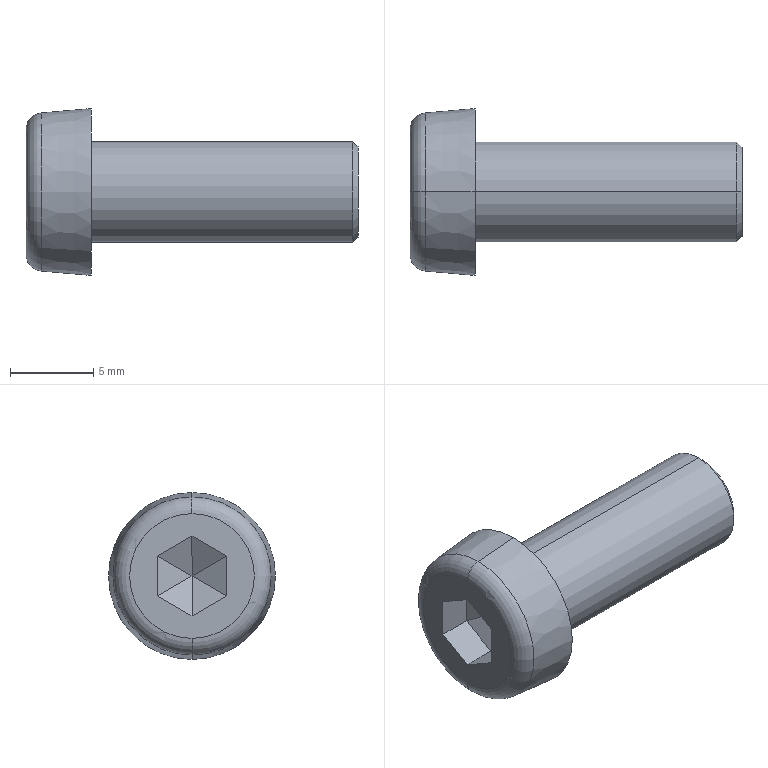Part | SolidWorks | features Cut 2, Fillet 2, Boss 1, Chamfer 1, Extrusion 1, LPattern 1, RevCut 1 | 1 solid | 23 faces | box 19.9 x 10 x 10 mm | volume 696.754 mm3 | plane 15 | cone 4 | torus 2 | cylinder 2 | commonest cylinder face diameters 6 x2
STEP:
#1=CARTESIAN_POINT('',(19.9,0.,-2.7));
#2=VERTEX_POINT('',#1);
#3=CARTESIAN_POINT('',(19.9,0.,2.7));
#4=VERTEX_POINT('',#3);
#5=CARTESIAN_POINT('',(19.9,0.,0.));
#6=DIRECTION('',(1.,0.,0.));
#7=DIRECTION('',(0.,0.,-1.));
#8=AXIS2_PLACEMENT_3D('',#5,#6,#7);
#9=CIRCLE('',#8,2.7);
#10=EDGE_CURVE('',#2,#4,#9,.T.);
#11=ORIENTED_EDGE('',*,*,#10,.F.);
#12=CARTESIAN_POINT('',(19.6,0.,-3.));
#13=VERTEX_POINT('',#12);
#14=CARTESIAN_POINT('',(19.9,0.,-2.7));
#15=DIRECTION('',(-0.7071,0.,-0.7071));
#16=VECTOR('',#15,1000.);
#17=LINE('',#14,#16);
#18=EDGE_CURVE('',#2,#13,#17,.T.);
#19=ORIENTED_EDGE('',*,*,#18,.T.);
#20=CARTESIAN_POINT('',(19.6,0.,3.));
#21=VERTEX_POINT('',#20);
#22=CARTESIAN_POINT('',(19.6,0.,0.));
#23=DIRECTION('',(-1.,0.,0.));
#24=DIRECTION('',(0.,0.,-1.));
#25=AXIS2_PLACEMENT_3D('',#22,#23,#24);
#26=CIRCLE('',#25,3.);
#27=EDGE_CURVE('',#21,#13,#26,.T.);
#28=ORIENTED_EDGE('',*,*,#27,.F.);
#29=CARTESIAN_POINT('',(19.9,0.,2.7));
#30=DIRECTION('',(-0.7071,0.,0.7071));
#31=VECTOR('',#30,1000.);
#32=LINE('',#29,#31);
#33=EDGE_CURVE('',#4,#21,#32,.T.);
#34=ORIENTED_EDGE('',*,*,#33,.F.);
#35=EDGE_LOOP('',(#11,#19,#28,#34));
#36=FACE_OUTER_BOUND('',#35,.T.);
#37=CARTESIAN_POINT('',(19.9,0.,0.));
#38=DIRECTION('',(-1.,0.,0.));
#39=DIRECTION('',(0.,0.,1.));
#40=AXIS2_PLACEMENT_3D('',#37,#38,#39);
#41=CONICAL_SURFACE('',#40,2.7,0.7854);
#42=ADVANCED_FACE('',(#36),#41,.T.);
#43=CARTESIAN_POINT('',(0.,0.,3.742));
#44=VERTEX_POINT('',#43);
#45=CARTESIAN_POINT('',(0.,0.,-3.742));
#46=VERTEX_POINT('',#45);
#47=CARTESIAN_POINT('',(0.,0.,0.));
#48=DIRECTION('',(-1.,0.,0.));
#49=DIRECTION('',(0.,0.,-1.));
#50=AXIS2_PLACEMENT_3D('',#47,#48,#49);
#51=CIRCLE('',#50,3.742);
#52=EDGE_CURVE('',#44,#46,#51,.T.);
#53=ORIENTED_EDGE('',*,*,#52,.F.);
#54=CARTESIAN_POINT('',(0.9128,0.,4.739));
#55=VERTEX_POINT('',#54);
#56=CARTESIAN_POINT('',(1.,0.,3.742));
#57=DIRECTION('',(0.,1.,0.));
#58=DIRECTION('',(0.,0.,1.));
#59=AXIS2_PLACEMENT_3D('',#56,#57,#58);
#60=CIRCLE('',#59,1.);
#61=EDGE_CURVE('',#44,#55,#60,.T.);
#62=ORIENTED_EDGE('',*,*,#61,.T.);
#63=CARTESIAN_POINT('',(0.9128,0.,-4.739));
#64=VERTEX_POINT('',#63);
#65=CARTESIAN_POINT('',(0.9128,0.,0.));
#66=DIRECTION('',(1.,0.,0.));
#67=DIRECTION('',(0.,0.,-1.));
#68=AXIS2_PLACEMENT_3D('',#65,#66,#67);
#69=CIRCLE('',#68,4.739);
#70=EDGE_CURVE('',#64,#55,#69,.T.);
#71=ORIENTED_EDGE('',*,*,#70,.F.);
#72=CARTESIAN_POINT('',(1.,0.,-3.742));
#73=DIRECTION('',(0.,-1.,0.));
#74=DIRECTION('',(0.,0.,-1.));
#75=AXIS2_PLACEMENT_3D('',#72,#73,#74);
#76=CIRCLE('',#75,1.);
#77=EDGE_CURVE('',#46,#64,#76,.T.);
#78=ORIENTED_EDGE('',*,*,#77,.F.);
#79=EDGE_LOOP('',(#53,#62,#71,#78));
#80=FACE_OUTER_BOUND('',#79,.T.);
#81=CARTESIAN_POINT('',(1.,0.,0.));
#82=DIRECTION('',(1.,0.,0.));
#83=DIRECTION('',(0.,0.,-1.));
#84=AXIS2_PLACEMENT_3D('',#81,#82,#83);
#85=TOROIDAL_SURFACE('',#84,3.742,1.);
#86=ADVANCED_FACE('',(#80),#85,.T.);
#87=ORIENTED_EDGE('',*,*,#27,.T.);
#88=CARTESIAN_POINT('',(3.9,0.,-3.));
#89=VERTEX_POINT('',#88);
#90=CARTESIAN_POINT('',(19.9,0.,-3.));
#91=DIRECTION('',(-1.,0.,0.));
#92=VECTOR('',#91,1000.);
#93=LINE('',#90,#92);
#94=EDGE_CURVE('',#13,#89,#93,.T.);
#95=ORIENTED_EDGE('',*,*,#94,.T.);
#96=CARTESIAN_POINT('',(3.9,0.,3.));
#97=VERTEX_POINT('',#96);
#98=CARTESIAN_POINT('',(3.9,0.,0.));
#99=DIRECTION('',(1.,0.,0.));
#100=DIRECTION('',(0.,0.,-1.));
#101=AXIS2_PLACEMENT_3D('',#98,#99,#100);
#102=CIRCLE('',#101,3.);
#103=EDGE_CURVE('',#89,#97,#102,.T.);
#104=ORIENTED_EDGE('',*,*,#103,.T.);
#105=CARTESIAN_POINT('',(19.9,0.,3.));
#106=DIRECTION('',(-1.,0.,0.));
#107=VECTOR('',#106,1000.);
#108=LINE('',#105,#107);
#109=EDGE_CURVE('',#21,#97,#108,.T.);
#110=ORIENTED_EDGE('',*,*,#109,.F.);
#111=EDGE_LOOP('',(#87,#95,#104,#110));
#112=FACE_OUTER_BOUND('',#111,.T.);
#113=CARTESIAN_POINT('',(19.9,0.,0.));
#114=DIRECTION('',(-1.,0.,0.));
#115=DIRECTION('',(0.,0.,1.));
#116=AXIS2_PLACEMENT_3D('',#113,#114,#115);
#117=CYLINDRICAL_SURFACE('',#116,3.);
#118=ADVANCED_FACE('',(#112),#117,.T.);
#119=ORIENTED_EDGE('',*,*,#70,.T.);
#120=CARTESIAN_POINT('',(3.9,0.,5.));
#121=VERTEX_POINT('',#120);
#122=CARTESIAN_POINT('',(3.9,0.,5.));
#123=DIRECTION('',(0.9962,0.,0.08716));
#124=VECTOR('',#123,1000.);
#125=LINE('',#122,#124);
#126=EDGE_CURVE('',#55,#121,#125,.T.);
#127=ORIENTED_EDGE('',*,*,#126,.T.);
#128=CARTESIAN_POINT('',(3.9,0.,-5.));
#129=VERTEX_POINT('',#128);
#130=CARTESIAN_POINT('',(3.9,0.,0.));
#131=DIRECTION('',(1.,0.,0.));
#132=DIRECTION('',(0.,0.,-1.));
#133=AXIS2_PLACEMENT_3D('',#130,#131,#132);
#134=CIRCLE('',#133,5.);
#135=EDGE_CURVE('',#129,#121,#134,.T.);
#136=ORIENTED_EDGE('',*,*,#135,.F.);
#137=CARTESIAN_POINT('',(3.9,0.,-5.));
#138=DIRECTION('',(0.9962,0.,-0.08716));
#139=VECTOR('',#138,1000.);
#140=LINE('',#137,#139);
#141=EDGE_CURVE('',#64,#129,#140,.T.);
#142=ORIENTED_EDGE('',*,*,#141,.F.);
#143=EDGE_LOOP('',(#119,#127,#136,#142));
#144=FACE_OUTER_BOUND('',#143,.T.);
#145=CARTESIAN_POINT('',(3.9,0.,0.));
#146=DIRECTION('',(1.,0.,0.));
#147=DIRECTION('',(0.,0.,-1.));
#148=AXIS2_PLACEMENT_3D('',#145,#146,#147);
#149=CONICAL_SURFACE('',#148,5.,0.08727);
#150=ADVANCED_FACE('',(#144),#149,.T.);
#151=CARTESIAN_POINT('',(0.,0.,0.));
#152=DIRECTION('',(-1.,0.,0.));
#153=DIRECTION('',(0.,0.,-1.));
#154=AXIS2_PLACEMENT_3D('',#151,#152,#153);
#155=CIRCLE('',#154,3.742);
#156=EDGE_CURVE('',#46,#44,#155,.T.);
#157=ORIENTED_EDGE('',*,*,#156,.T.);
#158=ORIENTED_EDGE('',*,*,#52,.T.);
#159=EDGE_LOOP('',(#157,#158));
#160=FACE_OUTER_BOUND('',#159,.T.);
#161=CARTESIAN_POINT('',(0.,-2.075,-1.198));
#162=VERTEX_POINT('',#161);
#163=CARTESIAN_POINT('',(0.,0.,-2.396));
#164=VERTEX_POINT('',#163);
#165=CARTESIAN_POINT('',(0.,-2.075,-1.198));
#166=DIRECTION('',(0.,0.866,-0.5));
#167=VECTOR('',#166,1000.);
#168=LINE('',#165,#167);
#169=EDGE_CURVE('',#162,#164,#168,.T.);
#170=ORIENTED_EDGE('',*,*,#169,.T.);
#171=CARTESIAN_POINT('',(0.,2.075,-1.198));
#172=VERTEX_POINT('',#171);
#173=CARTESIAN_POINT('',(0.,0.,-2.396));
#174=DIRECTION('',(0.,0.866,0.5));
#175=VECTOR('',#174,1000.);
#176=LINE('',#173,#175);
#177=EDGE_CURVE('',#164,#172,#176,.T.);
#178=ORIENTED_EDGE('',*,*,#177,.T.);
#179=CARTESIAN_POINT('',(0.,2.075,1.198));
#180=VERTEX_POINT('',#179);
#181=CARTESIAN_POINT('',(0.,2.075,-1.198));
#182=DIRECTION('',(0.,0.,1.));
#183=VECTOR('',#182,1000.);
#184=LINE('',#181,#183);
#185=EDGE_CURVE('',#172,#180,#184,.T.);
#186=ORIENTED_EDGE('',*,*,#185,.T.);
#187=CARTESIAN_POINT('',(0.,0.,2.396));
#188=VERTEX_POINT('',#187);
#189=CARTESIAN_POINT('',(0.,2.075,1.198));
#190=DIRECTION('',(0.,-0.866,0.5));
#191=VECTOR('',#190,1000.);
#192=LINE('',#189,#191);
#193=EDGE_CURVE('',#180,#188,#192,.T.);
#194=ORIENTED_EDGE('',*,*,#193,.T.);
#195=CARTESIAN_POINT('',(0.,-2.075,1.198));
#196=VERTEX_POINT('',#195);
#197=CARTESIAN_POINT('',(0.,0.,2.396));
#198=DIRECTION('',(0.,-0.866,-0.5));
#199=VECTOR('',#198,1000.);
#200=LINE('',#197,#199);
#201=EDGE_CURVE('',#188,#196,#200,.T.);
#202=ORIENTED_EDGE('',*,*,#201,.T.);
#203=CARTESIAN_POINT('',(0.,-2.075,1.198));
#204=DIRECTION('',(0.,0.,-1.));
#205=VECTOR('',#204,1000.);
#206=LINE('',#203,#205);
#207=EDGE_CURVE('',#196,#162,#206,.T.);
#208=ORIENTED_EDGE('',*,*,#207,.T.);
#209=EDGE_LOOP('',(#170,#178,#186,#194,#202,#208));
#210=FACE_BOUND('',#209,.T.);
#211=CARTESIAN_POINT('',(0.,0.,0.));
#212=DIRECTION('',(1.,0.,0.));
#213=DIRECTION('',(0.,0.,-1.));
#214=AXIS2_PLACEMENT_3D('',#211,#212,#213);
#215=PLANE('',#214);
#216=ADVANCED_FACE('',(#160,#210),#215,.F.);
#217=ORIENTED_EDGE('',*,*,#135,.T.);
#218=CARTESIAN_POINT('',(3.9,0.,0.));
#219=DIRECTION('',(1.,0.,0.));
#220=DIRECTION('',(0.,0.,-1.));
#221=AXIS2_PLACEMENT_3D('',#218,#219,#220);
#222=CIRCLE('',#221,5.);
#223=EDGE_CURVE('',#121,#129,#222,.T.);
#224=ORIENTED_EDGE('',*,*,#223,.T.);
#225=EDGE_LOOP('',(#217,#224));
#226=FACE_OUTER_BOUND('',#225,.T.);
#227=CARTESIAN_POINT('',(3.9,0.,0.));
#228=DIRECTION('',(1.,0.,0.));
#229=DIRECTION('',(0.,0.,-1.));
#230=AXIS2_PLACEMENT_3D('',#227,#228,#229);
#231=CIRCLE('',#230,3.);
#232=EDGE_CURVE('',#97,#89,#231,.T.);
#233=ORIENTED_EDGE('',*,*,#232,.F.);
#234=ORIENTED_EDGE('',*,*,#103,.F.);
#235=EDGE_LOOP('',(#233,#234));
#236=FACE_BOUND('',#235,.T.);
#237=CARTESIAN_POINT('',(3.9,0.,0.));
#238=DIRECTION('',(1.,0.,0.));
#239=DIRECTION('',(0.,0.,-1.));
#240=AXIS2_PLACEMENT_3D('',#237,#238,#239);
#241=PLANE('',#240);
#242=ADVANCED_FACE('',(#226,#236),#241,.T.);
#243=ORIENTED_EDGE('',*,*,#126,.F.);
#244=CARTESIAN_POINT('',(0.9128,0.,0.));
#245=DIRECTION('',(1.,0.,0.));
#246=DIRECTION('',(0.,0.,-1.));
#247=AXIS2_PLACEMENT_3D('',#244,#245,#246);
#248=CIRCLE('',#247,4.739);
#249=EDGE_CURVE('',#55,#64,#248,.T.);
#250=ORIENTED_EDGE('',*,*,#249,.T.);
#251=ORIENTED_EDGE('',*,*,#141,.T.);
#252=ORIENTED_EDGE('',*,*,#223,.F.);
#253=EDGE_LOOP('',(#243,#250,#251,#252));
#254=FACE_OUTER_BOUND('',#253,.T.);
#255=CARTESIAN_POINT('',(3.9,0.,0.));
#256=DIRECTION('',(1.,0.,0.));
#257=DIRECTION('',(0.,0.,-1.));
#258=AXIS2_PLACEMENT_3D('',#255,#256,#257);
#259=CONICAL_SURFACE('',#258,5.,0.08727);
#260=ADVANCED_FACE('',(#254),#259,.T.);
#261=ORIENTED_EDGE('',*,*,#94,.F.);
#262=CARTESIAN_POINT('',(19.6,0.,0.));
#263=DIRECTION('',(-1.,0.,0.));
#264=DIRECTION('',(0.,0.,-1.));
#265=AXIS2_PLACEMENT_3D('',#262,#263,#264);
#266=CIRCLE('',#265,3.);
#267=EDGE_CURVE('',#13,#21,#266,.T.);
#268=ORIENTED_EDGE('',*,*,#267,.T.);
#269=ORIENTED_EDGE('',*,*,#109,.T.);
#270=ORIENTED_EDGE('',*,*,#232,.T.);
#271=EDGE_LOOP('',(#261,#268,#269,#270));
#272=FACE_OUTER_BOUND('',#271,.T.);
#273=CARTESIAN_POINT('',(19.9,0.,0.));
#274=DIRECTION('',(-1.,0.,0.));
#275=DIRECTION('',(0.,0.,1.));
#276=AXIS2_PLACEMENT_3D('',#273,#274,#275);
#277=CYLINDRICAL_SURFACE('',#276,3.);
#278=ADVANCED_FACE('',(#272),#277,.T.);
#279=CARTESIAN_POINT('',(19.9,0.,0.));
#280=DIRECTION('',(1.,0.,0.));
#281=DIRECTION('',(0.,0.,-1.));
#282=AXIS2_PLACEMENT_3D('',#279,#280,#281);
#283=CIRCLE('',#282,2.7);
#284=EDGE_CURVE('',#4,#2,#283,.T.);
#285=ORIENTED_EDGE('',*,*,#284,.T.);
#286=ORIENTED_EDGE('',*,*,#10,.T.);
#287=EDGE_LOOP('',(#285,#286));
#288=FACE_OUTER_BOUND('',#287,.T.);
#289=CARTESIAN_POINT('',(19.9,0.,0.));
#290=DIRECTION('',(1.,0.,0.));
#291=DIRECTION('',(0.,0.,-1.));
#292=AXIS2_PLACEMENT_3D('',#289,#290,#291);
#293=PLANE('',#292);
#294=ADVANCED_FACE('',(#288),#293,.T.);
#295=ORIENTED_EDGE('',*,*,#169,.F.);
#296=CARTESIAN_POINT('',(2.,-2.075,-1.198));
#297=VERTEX_POINT('',#296);
#298=CARTESIAN_POINT('',(2.,-2.075,-1.198));
#299=DIRECTION('',(-1.,0.,0.));
#300=VECTOR('',#299,1000.);
#301=LINE('',#298,#300);
#302=EDGE_CURVE('',#297,#162,#301,.T.);
#303=ORIENTED_EDGE('',*,*,#302,.F.);
#304=CARTESIAN_POINT('',(2.,0.,-2.396));
#305=VERTEX_POINT('',#304);
#306=CARTESIAN_POINT('',(2.,-2.075,-1.198));
#307=DIRECTION('',(0.,0.866,-0.5));
#308=VECTOR('',#307,1000.);
#309=LINE('',#306,#308);
#310=EDGE_CURVE('',#297,#305,#309,.T.);
#311=ORIENTED_EDGE('',*,*,#310,.T.);
#312=CARTESIAN_POINT('',(2.,0.,-2.396));
#313=DIRECTION('',(-1.,0.,0.));
#314=VECTOR('',#313,1000.);
#315=LINE('',#312,#314);
#316=EDGE_CURVE('',#305,#164,#315,.T.);
#317=ORIENTED_EDGE('',*,*,#316,.T.);
#318=EDGE_LOOP('',(#295,#303,#311,#317));
#319=FACE_OUTER_BOUND('',#318,.T.);
#320=CARTESIAN_POINT('',(2.,-2.075,-1.198));
#321=DIRECTION('',(0.,0.5,0.866));
#322=DIRECTION('',(0.,-0.866,0.5));
#323=AXIS2_PLACEMENT_3D('',#320,#321,#322);
#324=PLANE('',#323);
#325=ADVANCED_FACE('',(#319),#324,.T.);
#326=ORIENTED_EDGE('',*,*,#177,.F.);
#327=ORIENTED_EDGE('',*,*,#316,.F.);
#328=CARTESIAN_POINT('',(2.,2.075,-1.198));
#329=VERTEX_POINT('',#328);
#330=CARTESIAN_POINT('',(2.,0.,-2.396));
#331=DIRECTION('',(0.,0.866,0.5));
#332=VECTOR('',#331,1000.);
#333=LINE('',#330,#332);
#334=EDGE_CURVE('',#305,#329,#333,.T.);
#335=ORIENTED_EDGE('',*,*,#334,.T.);
#336=CARTESIAN_POINT('',(2.,2.075,-1.198));
#337=DIRECTION('',(-1.,0.,0.));
#338=VECTOR('',#337,1000.);
#339=LINE('',#336,#338);
#340=EDGE_CURVE('',#329,#172,#339,.T.);
#341=ORIENTED_EDGE('',*,*,#340,.T.);
#342=EDGE_LOOP('',(#326,#327,#335,#341));
#343=FACE_OUTER_BOUND('',#342,.T.);
#344=CARTESIAN_POINT('',(2.,0.,-2.396));
#345=DIRECTION('',(0.,-0.5,0.866));
#346=DIRECTION('',(0.,-0.866,-0.5));
#347=AXIS2_PLACEMENT_3D('',#344,#345,#346);
#348=PLANE('',#347);
#349=ADVANCED_FACE('',(#343),#348,.T.);
#350=ORIENTED_EDGE('',*,*,#185,.F.);
#351=ORIENTED_EDGE('',*,*,#340,.F.);
#352=CARTESIAN_POINT('',(2.,2.075,1.198));
#353=VERTEX_POINT('',#352);
#354=CARTESIAN_POINT('',(2.,2.075,-1.198));
#355=DIRECTION('',(0.,0.,1.));
#356=VECTOR('',#355,1000.);
#357=LINE('',#354,#356);
#358=EDGE_CURVE('',#329,#353,#357,.T.);
#359=ORIENTED_EDGE('',*,*,#358,.T.);
#360=CARTESIAN_POINT('',(2.,2.075,1.198));
#361=DIRECTION('',(-1.,0.,0.));
#362=VECTOR('',#361,1000.);
#363=LINE('',#360,#362);
#364=EDGE_CURVE('',#353,#180,#363,.T.);
#365=ORIENTED_EDGE('',*,*,#364,.T.);
#366=EDGE_LOOP('',(#350,#351,#359,#365));
#367=FACE_OUTER_BOUND('',#366,.T.);
#368=CARTESIAN_POINT('',(2.,2.075,-1.198));
#369=DIRECTION('',(0.,-1.,0.));
#370=DIRECTION('',(0.,0.,-1.));
#371=AXIS2_PLACEMENT_3D('',#368,#369,#370);
#372=PLANE('',#371);
#373=ADVANCED_FACE('',(#367),#372,.T.);
#374=ORIENTED_EDGE('',*,*,#193,.F.);
#375=ORIENTED_EDGE('',*,*,#364,.F.);
#376=CARTESIAN_POINT('',(2.,0.,2.396));
#377=VERTEX_POINT('',#376);
#378=CARTESIAN_POINT('',(2.,2.075,1.198));
#379=DIRECTION('',(0.,-0.866,0.5));
#380=VECTOR('',#379,1000.);
#381=LINE('',#378,#380);
#382=EDGE_CURVE('',#353,#377,#381,.T.);
#383=ORIENTED_EDGE('',*,*,#382,.T.);
#384=CARTESIAN_POINT('',(2.,0.,2.396));
#385=DIRECTION('',(-1.,0.,0.));
#386=VECTOR('',#385,1000.);
#387=LINE('',#384,#386);
#388=EDGE_CURVE('',#377,#188,#387,.T.);
#389=ORIENTED_EDGE('',*,*,#388,.T.);
#390=EDGE_LOOP('',(#374,#375,#383,#389));
#391=FACE_OUTER_BOUND('',#390,.T.);
#392=CARTESIAN_POINT('',(2.,2.075,1.198));
#393=DIRECTION('',(0.,-0.5,-0.866));
#394=DIRECTION('',(0.,0.866,-0.5));
#395=AXIS2_PLACEMENT_3D('',#392,#393,#394);
#396=PLANE('',#395);
#397=ADVANCED_FACE('',(#391),#396,.T.);
#398=ORIENTED_EDGE('',*,*,#201,.F.);
#399=ORIENTED_EDGE('',*,*,#388,.F.);
#400=CARTESIAN_POINT('',(2.,-2.075,1.198));
#401=VERTEX_POINT('',#400);
#402=CARTESIAN_POINT('',(2.,0.,2.396));
#403=DIRECTION('',(0.,-0.866,-0.5));
#404=VECTOR('',#403,1000.);
#405=LINE('',#402,#404);
#406=EDGE_CURVE('',#377,#401,#405,.T.);
#407=ORIENTED_EDGE('',*,*,#406,.T.);
#408=CARTESIAN_POINT('',(2.,-2.075,1.198));
#409=DIRECTION('',(-1.,0.,0.));
#410=VECTOR('',#409,1000.);
#411=LINE('',#408,#410);
#412=EDGE_CURVE('',#401,#196,#411,.T.);
#413=ORIENTED_EDGE('',*,*,#412,.T.);
#414=EDGE_LOOP('',(#398,#399,#407,#413));
#415=FACE_OUTER_BOUND('',#414,.T.);
#416=CARTESIAN_POINT('',(2.,0.,2.396));
#417=DIRECTION('',(0.,0.5,-0.866));
#418=DIRECTION('',(0.,0.866,0.5));
#419=AXIS2_PLACEMENT_3D('',#416,#417,#418);
#420=PLANE('',#419);
#421=ADVANCED_FACE('',(#415),#420,.T.);
#422=ORIENTED_EDGE('',*,*,#207,.F.);
#423=ORIENTED_EDGE('',*,*,#412,.F.);
#424=CARTESIAN_POINT('',(2.,-2.075,1.198));
#425=DIRECTION('',(0.,0.,-1.));
#426=VECTOR('',#425,1000.);
#427=LINE('',#424,#426);
#428=EDGE_CURVE('',#401,#297,#427,.T.);
#429=ORIENTED_EDGE('',*,*,#428,.T.);
#430=ORIENTED_EDGE('',*,*,#302,.T.);
#431=EDGE_LOOP('',(#422,#423,#429,#430));
#432=FACE_OUTER_BOUND('',#431,.T.);
#433=CARTESIAN_POINT('',(2.,-2.075,1.198));
#434=DIRECTION('',(0.,1.,0.));
#435=DIRECTION('',(0.,0.,1.));
#436=AXIS2_PLACEMENT_3D('',#433,#434,#435);
#437=PLANE('',#436);
#438=ADVANCED_FACE('',(#432),#437,.T.);
#439=ORIENTED_EDGE('',*,*,#406,.F.);
#440=CARTESIAN_POINT('',(3.198,0.,0.));
#441=VERTEX_POINT('',#440);
#442=CARTESIAN_POINT('',(2.,0.,2.396));
#443=DIRECTION('',(-0.4472,0.,0.8944));
#444=VECTOR('',#443,1000.);
#445=LINE('',#442,#444);
#446=EDGE_CURVE('',#441,#377,#445,.T.);
#447=ORIENTED_EDGE('',*,*,#446,.F.);
#448=CARTESIAN_POINT('',(2.,-2.075,1.198));
#449=DIRECTION('',(-0.4472,-0.7746,0.4472));
#450=VECTOR('',#449,1000.);
#451=LINE('',#448,#450);
#452=EDGE_CURVE('',#441,#401,#451,.T.);
#453=ORIENTED_EDGE('',*,*,#452,.T.);
#454=EDGE_LOOP('',(#439,#447,#453));
#455=FACE_OUTER_BOUND('',#454,.T.);
#456=CARTESIAN_POINT('',(2.,0.,2.396));
#457=DIRECTION('',(0.866,-0.25,0.433));
#458=DIRECTION('',(0.4472,0.,-0.8944));
#459=AXIS2_PLACEMENT_3D('',#456,#457,#458);
#460=PLANE('',#459);
#461=ADVANCED_FACE('',(#455),#460,.F.);
#462=ORIENTED_EDGE('',*,*,#428,.F.);
#463=ORIENTED_EDGE('',*,*,#452,.F.);
#464=CARTESIAN_POINT('',(2.,-2.075,-1.198));
#465=DIRECTION('',(-0.4472,-0.7746,-0.4472));
#466=VECTOR('',#465,1000.);
#467=LINE('',#464,#466);
#468=EDGE_CURVE('',#441,#297,#467,.T.);
#469=ORIENTED_EDGE('',*,*,#468,.T.);
#470=EDGE_LOOP('',(#462,#463,#469));
#471=FACE_OUTER_BOUND('',#470,.T.);
#472=CARTESIAN_POINT('',(2.,-2.075,1.198));
#473=DIRECTION('',(0.866,-0.5,0.));
#474=DIRECTION('',(0.5,0.866,0.));
#475=AXIS2_PLACEMENT_3D('',#472,#473,#474);
#476=PLANE('',#475);
#477=ADVANCED_FACE('',(#471),#476,.F.);
#478=ORIENTED_EDGE('',*,*,#310,.F.);
#479=ORIENTED_EDGE('',*,*,#468,.F.);
#480=CARTESIAN_POINT('',(2.,0.,-2.396));
#481=DIRECTION('',(-0.4472,0.,-0.8944));
#482=VECTOR('',#481,1000.);
#483=LINE('',#480,#482);
#484=EDGE_CURVE('',#441,#305,#483,.T.);
#485=ORIENTED_EDGE('',*,*,#484,.T.);
#486=EDGE_LOOP('',(#478,#479,#485));
#487=FACE_OUTER_BOUND('',#486,.T.);
#488=CARTESIAN_POINT('',(2.,-2.075,-1.198));
#489=DIRECTION('',(0.866,-0.25,-0.433));
#490=DIRECTION('',(-0.4472,0.,-0.8944));
#491=AXIS2_PLACEMENT_3D('',#488,#489,#490);
#492=PLANE('',#491);
#493=ADVANCED_FACE('',(#487),#492,.F.);
#494=ORIENTED_EDGE('',*,*,#334,.F.);
#495=ORIENTED_EDGE('',*,*,#484,.F.);
#496=CARTESIAN_POINT('',(2.,2.075,-1.198));
#497=DIRECTION('',(-0.4472,0.7746,-0.4472));
#498=VECTOR('',#497,1000.);
#499=LINE('',#496,#498);
#500=EDGE_CURVE('',#441,#329,#499,.T.);
#501=ORIENTED_EDGE('',*,*,#500,.T.);
#502=EDGE_LOOP('',(#494,#495,#501));
#503=FACE_OUTER_BOUND('',#502,.T.);
#504=CARTESIAN_POINT('',(2.,0.,-2.396));
#505=DIRECTION('',(0.866,0.25,-0.433));
#506=DIRECTION('',(-0.4472,0.,-0.8944));
#507=AXIS2_PLACEMENT_3D('',#504,#505,#506);
#508=PLANE('',#507);
#509=ADVANCED_FACE('',(#503),#508,.F.);
#510=ORIENTED_EDGE('',*,*,#358,.F.);
#511=ORIENTED_EDGE('',*,*,#500,.F.);
#512=CARTESIAN_POINT('',(2.,2.075,1.198));
#513=DIRECTION('',(-0.4472,0.7746,0.4472));
#514=VECTOR('',#513,1000.);
#515=LINE('',#512,#514);
#516=EDGE_CURVE('',#441,#353,#515,.T.);
#517=ORIENTED_EDGE('',*,*,#516,.T.);
#518=EDGE_LOOP('',(#510,#511,#517));
#519=FACE_OUTER_BOUND('',#518,.T.);
#520=CARTESIAN_POINT('',(2.,2.075,-1.198));
#521=DIRECTION('',(0.866,0.5,0.));
#522=DIRECTION('',(-0.5,0.866,0.));
#523=AXIS2_PLACEMENT_3D('',#520,#521,#522);
#524=PLANE('',#523);
#525=ADVANCED_FACE('',(#519),#524,.F.);
#526=ORIENTED_EDGE('',*,*,#382,.F.);
#527=ORIENTED_EDGE('',*,*,#516,.F.);
#528=ORIENTED_EDGE('',*,*,#446,.T.);
#529=EDGE_LOOP('',(#526,#527,#528));
#530=FACE_OUTER_BOUND('',#529,.T.);
#531=CARTESIAN_POINT('',(2.,2.075,1.198));
#532=DIRECTION('',(0.866,0.25,0.433));
#533=DIRECTION('',(0.4472,0.,-0.8944));
#534=AXIS2_PLACEMENT_3D('',#531,#532,#533);
#535=PLANE('',#534);
#536=ADVANCED_FACE('',(#530),#535,.F.);
#537=ORIENTED_EDGE('',*,*,#61,.F.);
#538=ORIENTED_EDGE('',*,*,#156,.F.);
#539=ORIENTED_EDGE('',*,*,#77,.T.);
#540=ORIENTED_EDGE('',*,*,#249,.F.);
#541=EDGE_LOOP('',(#537,#538,#539,#540));
#542=FACE_OUTER_BOUND('',#541,.T.);
#543=CARTESIAN_POINT('',(1.,0.,0.));
#544=DIRECTION('',(1.,0.,0.));
#545=DIRECTION('',(0.,0.,-1.));
#546=AXIS2_PLACEMENT_3D('',#543,#544,#545);
#547=TOROIDAL_SURFACE('',#546,3.742,1.);
#548=ADVANCED_FACE('',(#542),#547,.T.);
#549=ORIENTED_EDGE('',*,*,#18,.F.);
#550=ORIENTED_EDGE('',*,*,#284,.F.);
#551=ORIENTED_EDGE('',*,*,#33,.T.);
#552=ORIENTED_EDGE('',*,*,#267,.F.);
#553=EDGE_LOOP('',(#549,#550,#551,#552));
#554=FACE_OUTER_BOUND('',#553,.T.);
#555=CARTESIAN_POINT('',(19.9,0.,0.));
#556=DIRECTION('',(-1.,0.,0.));
#557=DIRECTION('',(0.,0.,1.));
#558=AXIS2_PLACEMENT_3D('',#555,#556,#557);
#559=CONICAL_SURFACE('',#558,2.7,0.7854);
#560=ADVANCED_FACE('',(#554),#559,.T.);
#561=CLOSED_SHELL('',(#42,#86,#118,#150,#216,#242,#260,#278,#294,#325,#349,#373,#397,#421,#438,#461,#477,#493,#509,#525,#536,#548,#560));
#562=MANIFOLD_SOLID_BREP('',#561);
#563=CARTESIAN_POINT('',(0.,0.,0.));
#564=DIRECTION('',(0.,0.,1.));
#565=DIRECTION('',(1.,0.,0.));
#566=AXIS2_PLACEMENT_3D('',#563,#564,#565);
#567=(LENGTH_UNIT()NAMED_UNIT(*)SI_UNIT(.MILLI.,.METRE.));
#568=UNCERTAINTY_MEASURE_WITH_UNIT(LENGTH_MEASURE(0.00001),#567,'','');
#569=(NAMED_UNIT(*)PLANE_ANGLE_UNIT()SI_UNIT($,.RADIAN.));
#570=(NAMED_UNIT(*)SI_UNIT($,.STERADIAN.)SOLID_ANGLE_UNIT());
#571=(GEOMETRIC_REPRESENTATION_CONTEXT(3)GLOBAL_UNCERTAINTY_ASSIGNED_CONTEXT((#568))GLOBAL_UNIT_ASSIGNED_CONTEXT((#567,#569,#570))REPRESENTATION_CONTEXT('',''));
#572=ADVANCED_BREP_SHAPE_REPRESENTATION('',(#562,#566),#571);